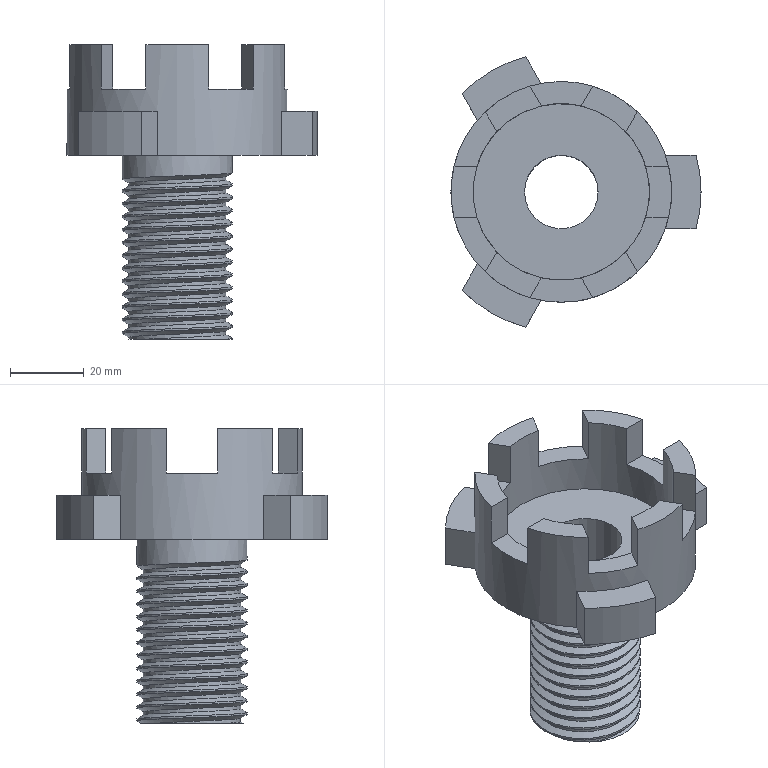Part | NX | features EXTRUDE 6, DATUM_CSYS 2, SKETCH 1, THREADS 1 | 1 solid | 59 faces | box 68 x 73.498 x 80 mm | volume 58295 mm3 | plane 37 | cylinder 20 | spline 2 | commonest cylinder face diameters 30 x13 76 x3 20 x1 26.5 x1 48 x1 60 x1